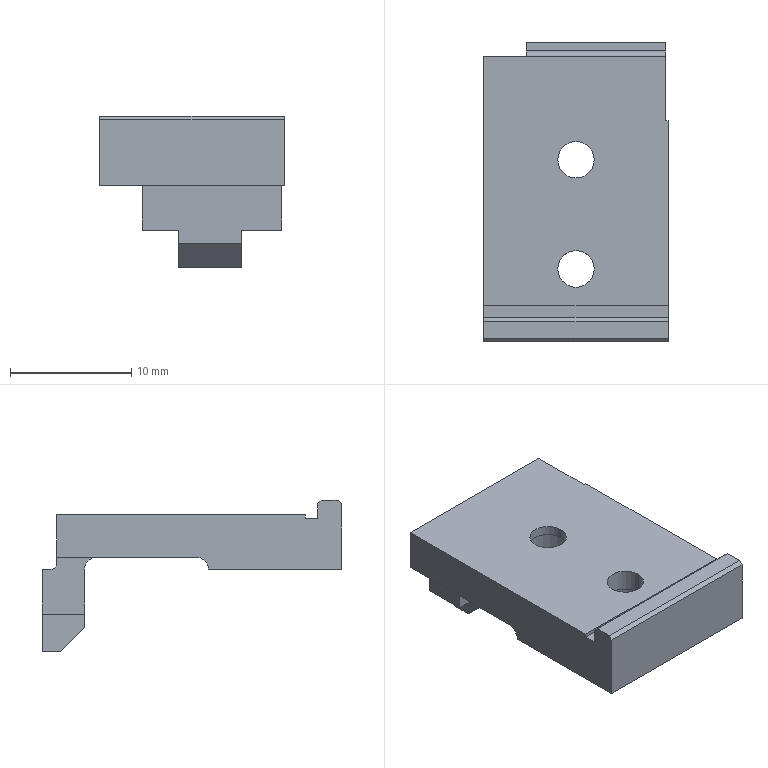Part | NX | 1 solid | 39 faces | box 15.2 x 24.7 x 12.5 mm | volume 1547 mm3 | plane 28 | cylinder 11 | commonest cylinder face diameters 3 x4 5 x4 2 x2 1 x1
STEP:
#1=CARTESIAN_POINT('',(-15.2,-12.7,1.));
#2=VERTEX_POINT('',#1);
#3=CARTESIAN_POINT('',(-15.2,-1.2,1.));
#4=VERTEX_POINT('',#3);
#5=CARTESIAN_POINT('',(-15.2,0.,1.));
#6=DIRECTION('',(0.,1.,0.));
#7=VECTOR('',#6,1000.);
#8=LINE('',#5,#7);
#9=EDGE_CURVE('',#2,#4,#8,.T.);
#10=ORIENTED_EDGE('',*,*,#9,.F.);
#11=CARTESIAN_POINT('',(-15.2,-13.7,0.));
#12=VERTEX_POINT('',#11);
#13=CARTESIAN_POINT('',(-15.2,-12.7,0.));
#14=DIRECTION('',(1.,0.,0.));
#15=DIRECTION('',(0.,-1.,0.));
#16=AXIS2_PLACEMENT_3D('',#13,#14,#15);
#17=CIRCLE('',#16,1.);
#18=EDGE_CURVE('',#2,#12,#17,.T.);
#19=ORIENTED_EDGE('',*,*,#18,.T.);
#20=CARTESIAN_POINT('',(-15.2,-24.7,0.));
#21=VERTEX_POINT('',#20);
#22=CARTESIAN_POINT('',(-15.2,0.,0.));
#23=DIRECTION('',(0.,1.,0.));
#24=VECTOR('',#23,1000.);
#25=LINE('',#22,#24);
#26=EDGE_CURVE('',#21,#12,#25,.T.);
#27=ORIENTED_EDGE('',*,*,#26,.F.);
#28=CARTESIAN_POINT('',(-15.2,-24.7,5.4));
#29=VERTEX_POINT('',#28);
#30=CARTESIAN_POINT('',(-15.2,-24.7,0.));
#31=DIRECTION('',(0.,0.,-1.));
#32=VECTOR('',#31,1000.);
#33=LINE('',#30,#32);
#34=EDGE_CURVE('',#29,#21,#33,.T.);
#35=ORIENTED_EDGE('',*,*,#34,.F.);
#36=CARTESIAN_POINT('',(-15.2,-24.4,5.7));
#37=VERTEX_POINT('',#36);
#38=CARTESIAN_POINT('',(-15.2,0.,30.1));
#39=DIRECTION('',(0.,0.7071,0.7071));
#40=VECTOR('',#39,1000.);
#41=LINE('',#38,#40);
#42=EDGE_CURVE('',#29,#37,#41,.T.);
#43=ORIENTED_EDGE('',*,*,#42,.T.);
#44=CARTESIAN_POINT('',(-15.2,-23.,5.7));
#45=VERTEX_POINT('',#44);
#46=CARTESIAN_POINT('',(-15.2,0.,5.7));
#47=DIRECTION('',(0.,1.,0.));
#48=VECTOR('',#47,1000.);
#49=LINE('',#46,#48);
#50=EDGE_CURVE('',#37,#45,#49,.T.);
#51=ORIENTED_EDGE('',*,*,#50,.T.);
#52=CARTESIAN_POINT('',(-15.2,-22.7,5.4));
#53=VERTEX_POINT('',#52);
#54=CARTESIAN_POINT('',(-15.2,0.,-17.3));
#55=DIRECTION('',(0.,-0.7071,0.7071));
#56=VECTOR('',#55,1000.);
#57=LINE('',#54,#56);
#58=EDGE_CURVE('',#53,#45,#57,.T.);
#59=ORIENTED_EDGE('',*,*,#58,.F.);
#60=CARTESIAN_POINT('',(-15.2,-22.7,4.2));
#61=VERTEX_POINT('',#60);
#62=CARTESIAN_POINT('',(-15.2,-22.7,0.));
#63=DIRECTION('',(0.,0.,-1.));
#64=VECTOR('',#63,1000.);
#65=LINE('',#62,#64);
#66=EDGE_CURVE('',#53,#61,#65,.T.);
#67=ORIENTED_EDGE('',*,*,#66,.T.);
#68=CARTESIAN_POINT('',(-15.2,-21.7,4.2));
#69=VERTEX_POINT('',#68);
#70=CARTESIAN_POINT('',(-15.2,0.,4.2));
#71=DIRECTION('',(0.,-1.,0.));
#72=VECTOR('',#71,1000.);
#73=LINE('',#70,#72);
#74=EDGE_CURVE('',#69,#61,#73,.T.);
#75=ORIENTED_EDGE('',*,*,#74,.F.);
#76=CARTESIAN_POINT('',(-15.2,-21.7,4.5));
#77=VERTEX_POINT('',#76);
#78=CARTESIAN_POINT('',(-15.2,-21.7,0.));
#79=DIRECTION('',(0.,0.,-1.));
#80=VECTOR('',#79,1000.);
#81=LINE('',#78,#80);
#82=EDGE_CURVE('',#77,#69,#81,.T.);
#83=ORIENTED_EDGE('',*,*,#82,.F.);
#84=CARTESIAN_POINT('',(-15.2,-1.2,4.5));
#85=VERTEX_POINT('',#84);
#86=CARTESIAN_POINT('',(-15.2,0.,4.5));
#87=DIRECTION('',(0.,-1.,0.));
#88=VECTOR('',#87,1000.);
#89=LINE('',#86,#88);
#90=EDGE_CURVE('',#85,#77,#89,.T.);
#91=ORIENTED_EDGE('',*,*,#90,.F.);
#92=CARTESIAN_POINT('',(-15.2,-1.2,0.));
#93=DIRECTION('',(0.,0.,1.));
#94=VECTOR('',#93,1000.);
#95=LINE('',#92,#94);
#96=EDGE_CURVE('',#4,#85,#95,.T.);
#97=ORIENTED_EDGE('',*,*,#96,.F.);
#98=EDGE_LOOP('',(#10,#19,#27,#35,#43,#51,#59,#67,#75,#83,#91,#97));
#99=FACE_BOUND('',#98,.T.);
#100=CARTESIAN_POINT('',(-15.2,0.,0.));
#101=DIRECTION('',(1.,0.,0.));
#102=DIRECTION('',(0.,1.,0.));
#103=AXIS2_PLACEMENT_3D('',#100,#101,#102);
#104=PLANE('',#103);
#105=ADVANCED_FACE('',(#99),#104,.F.);
#106=CARTESIAN_POINT('',(0.,-21.7,4.5));
#107=VERTEX_POINT('',#106);
#108=CARTESIAN_POINT('',(0.,-6.5,4.5));
#109=VERTEX_POINT('',#108);
#110=CARTESIAN_POINT('',(0.,0.,4.5));
#111=DIRECTION('',(0.,1.,0.));
#112=VECTOR('',#111,1000.);
#113=LINE('',#110,#112);
#114=EDGE_CURVE('',#107,#109,#113,.T.);
#115=ORIENTED_EDGE('',*,*,#114,.F.);
#116=CARTESIAN_POINT('',(0.,-21.7,4.2));
#117=VERTEX_POINT('',#116);
#118=CARTESIAN_POINT('',(0.,-21.7,0.));
#119=DIRECTION('',(0.,0.,1.));
#120=VECTOR('',#119,1000.);
#121=LINE('',#118,#120);
#122=EDGE_CURVE('',#117,#107,#121,.T.);
#123=ORIENTED_EDGE('',*,*,#122,.F.);
#124=CARTESIAN_POINT('',(0.,-22.7,4.2));
#125=VERTEX_POINT('',#124);
#126=CARTESIAN_POINT('',(0.,0.,4.2));
#127=DIRECTION('',(0.,1.,0.));
#128=VECTOR('',#127,1000.);
#129=LINE('',#126,#128);
#130=EDGE_CURVE('',#125,#117,#129,.T.);
#131=ORIENTED_EDGE('',*,*,#130,.F.);
#132=CARTESIAN_POINT('',(0.,-22.7,5.4));
#133=VERTEX_POINT('',#132);
#134=CARTESIAN_POINT('',(0.,-22.7,0.));
#135=DIRECTION('',(0.,0.,1.));
#136=VECTOR('',#135,1000.);
#137=LINE('',#134,#136);
#138=EDGE_CURVE('',#125,#133,#137,.T.);
#139=ORIENTED_EDGE('',*,*,#138,.T.);
#140=CARTESIAN_POINT('',(0.,-23.,5.7));
#141=VERTEX_POINT('',#140);
#142=CARTESIAN_POINT('',(0.,0.,-17.3));
#143=DIRECTION('',(0.,0.7071,-0.7071));
#144=VECTOR('',#143,1000.);
#145=LINE('',#142,#144);
#146=EDGE_CURVE('',#141,#133,#145,.T.);
#147=ORIENTED_EDGE('',*,*,#146,.F.);
#148=CARTESIAN_POINT('',(0.,-24.4,5.7));
#149=VERTEX_POINT('',#148);
#150=CARTESIAN_POINT('',(0.,0.,5.7));
#151=DIRECTION('',(0.,-1.,0.));
#152=VECTOR('',#151,1000.);
#153=LINE('',#150,#152);
#154=EDGE_CURVE('',#141,#149,#153,.T.);
#155=ORIENTED_EDGE('',*,*,#154,.T.);
#156=CARTESIAN_POINT('',(0.,-24.7,5.4));
#157=VERTEX_POINT('',#156);
#158=CARTESIAN_POINT('',(0.,0.,30.1));
#159=DIRECTION('',(0.,-0.7071,-0.7071));
#160=VECTOR('',#159,1000.);
#161=LINE('',#158,#160);
#162=EDGE_CURVE('',#149,#157,#161,.T.);
#163=ORIENTED_EDGE('',*,*,#162,.T.);
#164=CARTESIAN_POINT('',(0.,-24.7,0.));
#165=VERTEX_POINT('',#164);
#166=CARTESIAN_POINT('',(0.,-24.7,0.));
#167=DIRECTION('',(0.,0.,1.));
#168=VECTOR('',#167,1000.);
#169=LINE('',#166,#168);
#170=EDGE_CURVE('',#165,#157,#169,.T.);
#171=ORIENTED_EDGE('',*,*,#170,.F.);
#172=CARTESIAN_POINT('',(0.,-13.7,0.));
#173=VERTEX_POINT('',#172);
#174=CARTESIAN_POINT('',(0.,0.,0.));
#175=DIRECTION('',(0.,-1.,0.));
#176=VECTOR('',#175,1000.);
#177=LINE('',#174,#176);
#178=EDGE_CURVE('',#173,#165,#177,.T.);
#179=ORIENTED_EDGE('',*,*,#178,.F.);
#180=CARTESIAN_POINT('',(0.,-12.7,1.));
#181=VERTEX_POINT('',#180);
#182=CARTESIAN_POINT('',(0.,-12.7,0.));
#183=DIRECTION('',(1.,0.,0.));
#184=DIRECTION('',(0.,-1.,0.));
#185=AXIS2_PLACEMENT_3D('',#182,#183,#184);
#186=CIRCLE('',#185,1.);
#187=EDGE_CURVE('',#181,#173,#186,.T.);
#188=ORIENTED_EDGE('',*,*,#187,.F.);
#189=CARTESIAN_POINT('',(0.,-6.5,1.));
#190=VERTEX_POINT('',#189);
#191=CARTESIAN_POINT('',(0.,0.,1.));
#192=DIRECTION('',(0.,-1.,0.));
#193=VECTOR('',#192,1000.);
#194=LINE('',#191,#193);
#195=EDGE_CURVE('',#190,#181,#194,.T.);
#196=ORIENTED_EDGE('',*,*,#195,.F.);
#197=CARTESIAN_POINT('',(0.,-6.5,0.));
#198=DIRECTION('',(0.,0.,-1.));
#199=VECTOR('',#198,1000.);
#200=LINE('',#197,#199);
#201=EDGE_CURVE('',#109,#190,#200,.T.);
#202=ORIENTED_EDGE('',*,*,#201,.F.);
#203=EDGE_LOOP('',(#115,#123,#131,#139,#147,#155,#163,#171,#179,#188,#196,#202));
#204=FACE_BOUND('',#203,.T.);
#205=CARTESIAN_POINT('',(0.,-24.7,0.));
#206=DIRECTION('',(-1.,0.,0.));
#207=DIRECTION('',(0.,0.,1.));
#208=AXIS2_PLACEMENT_3D('',#205,#206,#207);
#209=PLANE('',#208);
#210=ADVANCED_FACE('',(#204),#209,.F.);
#211=CARTESIAN_POINT('',(-0.2,-1.2,4.5));
#212=VERTEX_POINT('',#211);
#213=CARTESIAN_POINT('',(-0.2,-6.5,4.5));
#214=VERTEX_POINT('',#213);
#215=CARTESIAN_POINT('',(-0.2,0.,4.5));
#216=DIRECTION('',(0.,-1.,0.));
#217=VECTOR('',#216,1000.);
#218=LINE('',#215,#217);
#219=EDGE_CURVE('',#212,#214,#218,.T.);
#220=ORIENTED_EDGE('',*,*,#219,.F.);
#221=CARTESIAN_POINT('',(0.,-1.2,4.5));
#222=DIRECTION('',(1.,0.,0.));
#223=VECTOR('',#222,1000.);
#224=LINE('',#221,#223);
#225=EDGE_CURVE('',#85,#212,#224,.T.);
#226=ORIENTED_EDGE('',*,*,#225,.F.);
#227=ORIENTED_EDGE('',*,*,#90,.T.);
#228=CARTESIAN_POINT('',(0.,-21.7,4.5));
#229=DIRECTION('',(-1.,0.,0.));
#230=VECTOR('',#229,1000.);
#231=LINE('',#228,#230);
#232=EDGE_CURVE('',#107,#77,#231,.T.);
#233=ORIENTED_EDGE('',*,*,#232,.F.);
#234=ORIENTED_EDGE('',*,*,#114,.T.);
#235=CARTESIAN_POINT('',(0.,-6.5,4.5));
#236=DIRECTION('',(1.,0.,0.));
#237=VECTOR('',#236,1000.);
#238=LINE('',#235,#237);
#239=EDGE_CURVE('',#214,#109,#238,.T.);
#240=ORIENTED_EDGE('',*,*,#239,.F.);
#241=EDGE_LOOP('',(#220,#226,#227,#233,#234,#240));
#242=FACE_BOUND('',#241,.T.);
#243=CARTESIAN_POINT('',(-6.1,-9.7,4.5));
#244=VERTEX_POINT('',#243);
#245=CARTESIAN_POINT('',(-9.1,-9.7,4.5));
#246=VERTEX_POINT('',#245);
#247=CARTESIAN_POINT('',(-7.6,-9.7,4.5));
#248=DIRECTION('',(0.,0.,-1.));
#249=DIRECTION('',(-1.,0.,0.));
#250=AXIS2_PLACEMENT_3D('',#247,#248,#249);
#251=CIRCLE('',#250,1.5);
#252=EDGE_CURVE('',#244,#246,#251,.T.);
#253=ORIENTED_EDGE('',*,*,#252,.T.);
#254=CARTESIAN_POINT('',(-7.6,-9.7,4.5));
#255=DIRECTION('',(0.,0.,-1.));
#256=DIRECTION('',(-1.,0.,0.));
#257=AXIS2_PLACEMENT_3D('',#254,#255,#256);
#258=CIRCLE('',#257,1.5);
#259=EDGE_CURVE('',#246,#244,#258,.T.);
#260=ORIENTED_EDGE('',*,*,#259,.T.);
#261=EDGE_LOOP('',(#253,#260));
#262=FACE_BOUND('',#261,.T.);
#263=CARTESIAN_POINT('',(-9.1,-18.7,4.5));
#264=VERTEX_POINT('',#263);
#265=CARTESIAN_POINT('',(-6.1,-18.7,4.5));
#266=VERTEX_POINT('',#265);
#267=CARTESIAN_POINT('',(-7.6,-18.7,4.5));
#268=DIRECTION('',(0.,0.,-1.));
#269=DIRECTION('',(-1.,0.,0.));
#270=AXIS2_PLACEMENT_3D('',#267,#268,#269);
#271=CIRCLE('',#270,1.5);
#272=EDGE_CURVE('',#264,#266,#271,.T.);
#273=ORIENTED_EDGE('',*,*,#272,.T.);
#274=CARTESIAN_POINT('',(-7.6,-18.7,4.5));
#275=DIRECTION('',(0.,0.,-1.));
#276=DIRECTION('',(-1.,0.,0.));
#277=AXIS2_PLACEMENT_3D('',#274,#275,#276);
#278=CIRCLE('',#277,1.5);
#279=EDGE_CURVE('',#266,#264,#278,.T.);
#280=ORIENTED_EDGE('',*,*,#279,.T.);
#281=EDGE_LOOP('',(#273,#280));
#282=FACE_BOUND('',#281,.T.);
#283=CARTESIAN_POINT('',(0.,0.,4.5));
#284=DIRECTION('',(0.,0.,1.));
#285=DIRECTION('',(1.,0.,0.));
#286=AXIS2_PLACEMENT_3D('',#283,#284,#285);
#287=PLANE('',#286);
#288=ADVANCED_FACE('',(#242,#262,#282),#287,.T.);
#289=CARTESIAN_POINT('',(-0.2,-4.5,1.));
#290=VERTEX_POINT('',#289);
#291=CARTESIAN_POINT('',(-11.7,-4.5,1.));
#292=VERTEX_POINT('',#291);
#293=CARTESIAN_POINT('',(0.,-4.5,1.));
#294=DIRECTION('',(-1.,0.,0.));
#295=VECTOR('',#294,1000.);
#296=LINE('',#293,#295);
#297=EDGE_CURVE('',#290,#292,#296,.T.);
#298=ORIENTED_EDGE('',*,*,#297,.F.);
#299=CARTESIAN_POINT('',(-0.2,-6.5,1.));
#300=VERTEX_POINT('',#299);
#301=CARTESIAN_POINT('',(-0.2,0.,1.));
#302=DIRECTION('',(0.,-1.,0.));
#303=VECTOR('',#302,1000.);
#304=LINE('',#301,#303);
#305=EDGE_CURVE('',#290,#300,#304,.T.);
#306=ORIENTED_EDGE('',*,*,#305,.T.);
#307=CARTESIAN_POINT('',(0.,-6.5,1.));
#308=DIRECTION('',(-1.,0.,0.));
#309=VECTOR('',#308,1000.);
#310=LINE('',#307,#309);
#311=EDGE_CURVE('',#190,#300,#310,.T.);
#312=ORIENTED_EDGE('',*,*,#311,.F.);
#313=ORIENTED_EDGE('',*,*,#195,.T.);
#314=CARTESIAN_POINT('',(0.,-12.7,1.));
#315=DIRECTION('',(1.,0.,0.));
#316=VECTOR('',#315,1000.);
#317=LINE('',#314,#316);
#318=EDGE_CURVE('',#2,#181,#317,.T.);
#319=ORIENTED_EDGE('',*,*,#318,.F.);
#320=ORIENTED_EDGE('',*,*,#9,.T.);
#321=CARTESIAN_POINT('',(-11.7,-1.2,1.));
#322=VERTEX_POINT('',#321);
#323=CARTESIAN_POINT('',(0.,-1.2,1.));
#324=DIRECTION('',(-1.,0.,0.));
#325=VECTOR('',#324,1000.);
#326=LINE('',#323,#325);
#327=EDGE_CURVE('',#322,#4,#326,.T.);
#328=ORIENTED_EDGE('',*,*,#327,.F.);
#329=CARTESIAN_POINT('',(-11.7,0.,1.));
#330=DIRECTION('',(0.,-1.,0.));
#331=VECTOR('',#330,1000.);
#332=LINE('',#329,#331);
#333=EDGE_CURVE('',#322,#292,#332,.T.);
#334=ORIENTED_EDGE('',*,*,#333,.T.);
#335=EDGE_LOOP('',(#298,#306,#312,#313,#319,#320,#328,#334));
#336=FACE_BOUND('',#335,.T.);
#337=CARTESIAN_POINT('',(-5.1,-9.7,1.));
#338=VERTEX_POINT('',#337);
#339=CARTESIAN_POINT('',(-10.1,-9.7,1.));
#340=VERTEX_POINT('',#339);
#341=CARTESIAN_POINT('',(-7.6,-9.7,1.));
#342=DIRECTION('',(0.,0.,-1.));
#343=DIRECTION('',(-1.,0.,0.));
#344=AXIS2_PLACEMENT_3D('',#341,#342,#343);
#345=CIRCLE('',#344,2.5);
#346=EDGE_CURVE('',#338,#340,#345,.T.);
#347=ORIENTED_EDGE('',*,*,#346,.F.);
#348=CARTESIAN_POINT('',(-7.6,-9.7,1.));
#349=DIRECTION('',(0.,0.,-1.));
#350=DIRECTION('',(-1.,0.,0.));
#351=AXIS2_PLACEMENT_3D('',#348,#349,#350);
#352=CIRCLE('',#351,2.5);
#353=EDGE_CURVE('',#340,#338,#352,.T.);
#354=ORIENTED_EDGE('',*,*,#353,.F.);
#355=EDGE_LOOP('',(#347,#354));
#356=FACE_BOUND('',#355,.T.);
#357=CARTESIAN_POINT('',(-11.724,-4.43,1.));
#358=DIRECTION('',(0.,0.,-1.));
#359=DIRECTION('',(0.,-1.,0.));
#360=AXIS2_PLACEMENT_3D('',#357,#358,#359);
#361=PLANE('',#360);
#362=ADVANCED_FACE('',(#336,#356),#361,.T.);
#363=CARTESIAN_POINT('',(-0.2,-3.5,-3.7));
#364=VERTEX_POINT('',#363);
#365=CARTESIAN_POINT('',(-0.2,0.,-3.7));
#366=VERTEX_POINT('',#365);
#367=CARTESIAN_POINT('',(-0.2,0.,-3.7));
#368=DIRECTION('',(0.,1.,0.));
#369=VECTOR('',#368,1000.);
#370=LINE('',#367,#369);
#371=EDGE_CURVE('',#364,#366,#370,.T.);
#372=ORIENTED_EDGE('',*,*,#371,.T.);
#373=CARTESIAN_POINT('',(-0.2,0.,0.));
#374=VERTEX_POINT('',#373);
#375=CARTESIAN_POINT('',(-0.2,0.,0.));
#376=DIRECTION('',(0.,0.,-1.));
#377=VECTOR('',#376,1000.);
#378=LINE('',#375,#377);
#379=EDGE_CURVE('',#374,#366,#378,.T.);
#380=ORIENTED_EDGE('',*,*,#379,.F.);
#381=CARTESIAN_POINT('',(-0.2,-0.7,0.));
#382=VERTEX_POINT('',#381);
#383=CARTESIAN_POINT('',(-0.2,0.,0.));
#384=DIRECTION('',(0.,1.,0.));
#385=VECTOR('',#384,1000.);
#386=LINE('',#383,#385);
#387=EDGE_CURVE('',#382,#374,#386,.T.);
#388=ORIENTED_EDGE('',*,*,#387,.F.);
#389=CARTESIAN_POINT('',(-0.2,-1.2,0.5));
#390=VERTEX_POINT('',#389);
#391=CARTESIAN_POINT('',(-0.2,-0.7,0.5));
#392=DIRECTION('',(-1.,0.,0.));
#393=DIRECTION('',(0.,1.,0.));
#394=AXIS2_PLACEMENT_3D('',#391,#392,#393);
#395=CIRCLE('',#394,0.5);
#396=EDGE_CURVE('',#382,#390,#395,.T.);
#397=ORIENTED_EDGE('',*,*,#396,.T.);
#398=CARTESIAN_POINT('',(-0.2,-1.2,0.));
#399=DIRECTION('',(0.,0.,-1.));
#400=VECTOR('',#399,1000.);
#401=LINE('',#398,#400);
#402=EDGE_CURVE('',#212,#390,#401,.T.);
#403=ORIENTED_EDGE('',*,*,#402,.F.);
#404=ORIENTED_EDGE('',*,*,#219,.T.);
#405=CARTESIAN_POINT('',(-0.2,-6.5,0.));
#406=DIRECTION('',(0.,0.,-1.));
#407=VECTOR('',#406,1000.);
#408=LINE('',#405,#407);
#409=EDGE_CURVE('',#214,#300,#408,.T.);
#410=ORIENTED_EDGE('',*,*,#409,.T.);
#411=ORIENTED_EDGE('',*,*,#305,.F.);
#412=CARTESIAN_POINT('',(-0.2,-3.5,0.));
#413=VERTEX_POINT('',#412);
#414=CARTESIAN_POINT('',(-0.2,-4.5,0.));
#415=DIRECTION('',(-1.,0.,0.));
#416=DIRECTION('',(0.,1.,0.));
#417=AXIS2_PLACEMENT_3D('',#414,#415,#416);
#418=CIRCLE('',#417,1.);
#419=EDGE_CURVE('',#290,#413,#418,.T.);
#420=ORIENTED_EDGE('',*,*,#419,.T.);
#421=CARTESIAN_POINT('',(-0.2,-3.5,0.));
#422=DIRECTION('',(0.,0.,1.));
#423=VECTOR('',#422,1000.);
#424=LINE('',#421,#423);
#425=EDGE_CURVE('',#364,#413,#424,.T.);
#426=ORIENTED_EDGE('',*,*,#425,.F.);
#427=EDGE_LOOP('',(#372,#380,#388,#397,#403,#404,#410,#411,#420,#426));
#428=FACE_BOUND('',#427,.T.);
#429=CARTESIAN_POINT('',(-0.2,-6.5,2.));
#430=DIRECTION('',(1.,0.,0.));
#431=DIRECTION('',(0.,1.,0.));
#432=AXIS2_PLACEMENT_3D('',#429,#430,#431);
#433=PLANE('',#432);
#434=ADVANCED_FACE('',(#428),#433,.T.);
#435=ORIENTED_EDGE('',*,*,#82,.T.);
#436=CARTESIAN_POINT('',(0.,-21.7,4.2));
#437=DIRECTION('',(1.,0.,0.));
#438=VECTOR('',#437,1000.);
#439=LINE('',#436,#438);
#440=EDGE_CURVE('',#69,#117,#439,.T.);
#441=ORIENTED_EDGE('',*,*,#440,.T.);
#442=ORIENTED_EDGE('',*,*,#122,.T.);
#443=ORIENTED_EDGE('',*,*,#232,.T.);
#444=EDGE_LOOP('',(#435,#441,#442,#443));
#445=FACE_BOUND('',#444,.T.);
#446=CARTESIAN_POINT('',(0.,-21.7,2.));
#447=DIRECTION('',(0.,-1.,0.));
#448=DIRECTION('',(0.,0.,-1.));
#449=AXIS2_PLACEMENT_3D('',#446,#447,#448);
#450=PLANE('',#449);
#451=ADVANCED_FACE('',(#445),#450,.T.);
#452=CARTESIAN_POINT('',(-11.7,0.,-3.7));
#453=VERTEX_POINT('',#452);
#454=CARTESIAN_POINT('',(-11.7,-3.5,-3.7));
#455=VERTEX_POINT('',#454);
#456=CARTESIAN_POINT('',(-11.7,0.,-3.7));
#457=DIRECTION('',(0.,-1.,0.));
#458=VECTOR('',#457,1000.);
#459=LINE('',#456,#458);
#460=EDGE_CURVE('',#453,#455,#459,.T.);
#461=ORIENTED_EDGE('',*,*,#460,.T.);
#462=CARTESIAN_POINT('',(-11.7,-3.5,0.));
#463=VERTEX_POINT('',#462);
#464=CARTESIAN_POINT('',(-11.7,-3.5,0.));
#465=DIRECTION('',(0.,0.,1.));
#466=VECTOR('',#465,1000.);
#467=LINE('',#464,#466);
#468=EDGE_CURVE('',#455,#463,#467,.T.);
#469=ORIENTED_EDGE('',*,*,#468,.T.);
#470=CARTESIAN_POINT('',(-11.7,-4.5,0.));
#471=DIRECTION('',(-1.,0.,0.));
#472=DIRECTION('',(0.,1.,0.));
#473=AXIS2_PLACEMENT_3D('',#470,#471,#472);
#474=CIRCLE('',#473,1.);
#475=EDGE_CURVE('',#292,#463,#474,.T.);
#476=ORIENTED_EDGE('',*,*,#475,.F.);
#477=ORIENTED_EDGE('',*,*,#333,.F.);
#478=CARTESIAN_POINT('',(-11.7,-1.2,0.5));
#479=VERTEX_POINT('',#478);
#480=CARTESIAN_POINT('',(-11.7,-1.2,0.));
#481=DIRECTION('',(0.,0.,-1.));
#482=VECTOR('',#481,1000.);
#483=LINE('',#480,#482);
#484=EDGE_CURVE('',#322,#479,#483,.T.);
#485=ORIENTED_EDGE('',*,*,#484,.T.);
#486=CARTESIAN_POINT('',(-11.7,-0.7,0.));
#487=VERTEX_POINT('',#486);
#488=CARTESIAN_POINT('',(-11.7,-0.7,0.5));
#489=DIRECTION('',(-1.,0.,0.));
#490=DIRECTION('',(0.,1.,0.));
#491=AXIS2_PLACEMENT_3D('',#488,#489,#490);
#492=CIRCLE('',#491,0.5);
#493=EDGE_CURVE('',#487,#479,#492,.T.);
#494=ORIENTED_EDGE('',*,*,#493,.F.);
#495=CARTESIAN_POINT('',(-11.7,0.,0.));
#496=VERTEX_POINT('',#495);
#497=CARTESIAN_POINT('',(-11.7,0.,0.));
#498=DIRECTION('',(0.,1.,0.));
#499=VECTOR('',#498,1000.);
#500=LINE('',#497,#499);
#501=EDGE_CURVE('',#487,#496,#500,.T.);
#502=ORIENTED_EDGE('',*,*,#501,.T.);
#503=CARTESIAN_POINT('',(-11.7,0.,0.));
#504=DIRECTION('',(0.,0.,-1.));
#505=VECTOR('',#504,1000.);
#506=LINE('',#503,#505);
#507=EDGE_CURVE('',#496,#453,#506,.T.);
#508=ORIENTED_EDGE('',*,*,#507,.T.);
#509=EDGE_LOOP('',(#461,#469,#476,#477,#485,#494,#502,#508));
#510=FACE_BOUND('',#509,.T.);
#511=CARTESIAN_POINT('',(-11.7,-1.2,0.));
#512=DIRECTION('',(1.,0.,0.));
#513=DIRECTION('',(0.,1.,0.));
#514=AXIS2_PLACEMENT_3D('',#511,#512,#513);
#515=PLANE('',#514);
#516=ADVANCED_FACE('',(#510),#515,.F.);
#517=ORIENTED_EDGE('',*,*,#311,.T.);
#518=ORIENTED_EDGE('',*,*,#409,.F.);
#519=ORIENTED_EDGE('',*,*,#239,.T.);
#520=ORIENTED_EDGE('',*,*,#201,.T.);
#521=EDGE_LOOP('',(#517,#518,#519,#520));
#522=FACE_BOUND('',#521,.T.);
#523=CARTESIAN_POINT('',(0.,-6.5,2.));
#524=DIRECTION('',(0.,1.,0.));
#525=DIRECTION('',(1.,0.,0.));
#526=AXIS2_PLACEMENT_3D('',#523,#524,#525);
#527=PLANE('',#526);
#528=ADVANCED_FACE('',(#522),#527,.T.);
#529=CARTESIAN_POINT('',(-5.1,-18.7,2.7));
#530=VERTEX_POINT('',#529);
#531=CARTESIAN_POINT('',(-10.1,-18.7,2.7));
#532=VERTEX_POINT('',#531);
#533=CARTESIAN_POINT('',(-7.6,-18.7,2.7));
#534=DIRECTION('',(0.,0.,-1.));
#535=DIRECTION('',(-1.,0.,0.));
#536=AXIS2_PLACEMENT_3D('',#533,#534,#535);
#537=CIRCLE('',#536,2.5);
#538=EDGE_CURVE('',#530,#532,#537,.T.);
#539=ORIENTED_EDGE('',*,*,#538,.T.);
#540=CARTESIAN_POINT('',(-7.6,-18.7,2.7));
#541=DIRECTION('',(0.,0.,-1.));
#542=DIRECTION('',(-1.,0.,0.));
#543=AXIS2_PLACEMENT_3D('',#540,#541,#542);
#544=CIRCLE('',#543,2.5);
#545=EDGE_CURVE('',#532,#530,#544,.T.);
#546=ORIENTED_EDGE('',*,*,#545,.T.);
#547=EDGE_LOOP('',(#539,#546));
#548=FACE_BOUND('',#547,.T.);
#549=CARTESIAN_POINT('',(-6.1,-18.7,2.7));
#550=VERTEX_POINT('',#549);
#551=CARTESIAN_POINT('',(-9.1,-18.7,2.7));
#552=VERTEX_POINT('',#551);
#553=CARTESIAN_POINT('',(-7.6,-18.7,2.7));
#554=DIRECTION('',(0.,0.,-1.));
#555=DIRECTION('',(-1.,0.,0.));
#556=AXIS2_PLACEMENT_3D('',#553,#554,#555);
#557=CIRCLE('',#556,1.5);
#558=EDGE_CURVE('',#550,#552,#557,.T.);
#559=ORIENTED_EDGE('',*,*,#558,.F.);
#560=CARTESIAN_POINT('',(-7.6,-18.7,2.7));
#561=DIRECTION('',(0.,0.,-1.));
#562=DIRECTION('',(-1.,0.,0.));
#563=AXIS2_PLACEMENT_3D('',#560,#561,#562);
#564=CIRCLE('',#563,1.5);
#565=EDGE_CURVE('',#552,#550,#564,.T.);
#566=ORIENTED_EDGE('',*,*,#565,.F.);
#567=EDGE_LOOP('',(#559,#566));
#568=FACE_BOUND('',#567,.T.);
#569=CARTESIAN_POINT('',(-11.486,-5.492,2.7));
#570=DIRECTION('',(0.,0.,-1.));
#571=DIRECTION('',(0.,-1.,0.));
#572=AXIS2_PLACEMENT_3D('',#569,#570,#571);
#573=PLANE('',#572);
#574=ADVANCED_FACE('',(#548,#568),#573,.T.);
#575=ORIENTED_EDGE('',*,*,#387,.T.);
#576=CARTESIAN_POINT('',(0.,0.,0.));
#577=DIRECTION('',(1.,0.,0.));
#578=VECTOR('',#577,1000.);
#579=LINE('',#576,#578);
#580=EDGE_CURVE('',#496,#374,#579,.T.);
#581=ORIENTED_EDGE('',*,*,#580,.F.);
#582=ORIENTED_EDGE('',*,*,#501,.F.);
#583=CARTESIAN_POINT('',(0.,-0.7,0.));
#584=DIRECTION('',(-1.,0.,0.));
#585=VECTOR('',#584,1000.);
#586=LINE('',#583,#585);
#587=EDGE_CURVE('',#382,#487,#586,.T.);
#588=ORIENTED_EDGE('',*,*,#587,.F.);
#589=EDGE_LOOP('',(#575,#581,#582,#588));
#590=FACE_BOUND('',#589,.T.);
#591=CARTESIAN_POINT('',(-15.2,-1.2,0.));
#592=DIRECTION('',(0.,0.,1.));
#593=DIRECTION('',(1.,0.,0.));
#594=AXIS2_PLACEMENT_3D('',#591,#592,#593);
#595=PLANE('',#594);
#596=ADVANCED_FACE('',(#590),#595,.T.);
#597=CARTESIAN_POINT('',(-4.1,0.,-6.8));
#598=VERTEX_POINT('',#597);
#599=CARTESIAN_POINT('',(-4.1,0.,-3.7));
#600=VERTEX_POINT('',#599);
#601=CARTESIAN_POINT('',(-4.1,0.,0.));
#602=DIRECTION('',(0.,0.,1.));
#603=VECTOR('',#602,1000.);
#604=LINE('',#601,#603);
#605=EDGE_CURVE('',#598,#600,#604,.T.);
#606=ORIENTED_EDGE('',*,*,#605,.F.);
#607=CARTESIAN_POINT('',(-8.7,0.,-6.8));
#608=VERTEX_POINT('',#607);
#609=CARTESIAN_POINT('',(0.,0.,-6.8));
#610=DIRECTION('',(-1.,0.,0.));
#611=VECTOR('',#610,1000.);
#612=LINE('',#609,#611);
#613=EDGE_CURVE('',#598,#608,#612,.T.);
#614=ORIENTED_EDGE('',*,*,#613,.T.);
#615=CARTESIAN_POINT('',(-8.7,0.,-3.7));
#616=VERTEX_POINT('',#615);
#617=CARTESIAN_POINT('',(-8.7,0.,0.));
#618=DIRECTION('',(0.,0.,1.));
#619=VECTOR('',#618,1000.);
#620=LINE('',#617,#619);
#621=EDGE_CURVE('',#608,#616,#620,.T.);
#622=ORIENTED_EDGE('',*,*,#621,.T.);
#623=CARTESIAN_POINT('',(0.,0.,-3.7));
#624=DIRECTION('',(1.,0.,0.));
#625=VECTOR('',#624,1000.);
#626=LINE('',#623,#625);
#627=EDGE_CURVE('',#453,#616,#626,.T.);
#628=ORIENTED_EDGE('',*,*,#627,.F.);
#629=ORIENTED_EDGE('',*,*,#507,.F.);
#630=ORIENTED_EDGE('',*,*,#580,.T.);
#631=ORIENTED_EDGE('',*,*,#379,.T.);
#632=CARTESIAN_POINT('',(0.,0.,-3.7));
#633=DIRECTION('',(1.,0.,0.));
#634=VECTOR('',#633,1000.);
#635=LINE('',#632,#634);
#636=EDGE_CURVE('',#600,#366,#635,.T.);
#637=ORIENTED_EDGE('',*,*,#636,.F.);
#638=EDGE_LOOP('',(#606,#614,#622,#628,#629,#630,#631,#637));
#639=FACE_BOUND('',#638,.T.);
#640=CARTESIAN_POINT('',(0.,0.,0.));
#641=DIRECTION('',(0.,-1.,0.));
#642=DIRECTION('',(0.,0.,-1.));
#643=AXIS2_PLACEMENT_3D('',#640,#641,#642);
#644=PLANE('',#643);
#645=ADVANCED_FACE('',(#639),#644,.F.);
#646=CARTESIAN_POINT('',(-8.7,-3.5,-3.7));
#647=VERTEX_POINT('',#646);
#648=CARTESIAN_POINT('',(-8.7,-3.5,-4.8));
#649=VERTEX_POINT('',#648);
#650=CARTESIAN_POINT('',(-8.7,-3.5,0.));
#651=DIRECTION('',(0.,0.,-1.));
#652=VECTOR('',#651,1000.);
#653=LINE('',#650,#652);
#654=EDGE_CURVE('',#647,#649,#653,.T.);
#655=ORIENTED_EDGE('',*,*,#654,.F.);
#656=CARTESIAN_POINT('',(-8.7,0.,-3.7));
#657=DIRECTION('',(0.,1.,0.));
#658=VECTOR('',#657,1000.);
#659=LINE('',#656,#658);
#660=EDGE_CURVE('',#647,#616,#659,.T.);
#661=ORIENTED_EDGE('',*,*,#660,.T.);
#662=ORIENTED_EDGE('',*,*,#621,.F.);
#663=CARTESIAN_POINT('',(-8.7,-1.5,-6.8));
#664=VERTEX_POINT('',#663);
#665=CARTESIAN_POINT('',(-8.7,0.,-6.8));
#666=DIRECTION('',(0.,1.,0.));
#667=VECTOR('',#666,1000.);
#668=LINE('',#665,#667);
#669=EDGE_CURVE('',#664,#608,#668,.T.);
#670=ORIENTED_EDGE('',*,*,#669,.F.);
#671=CARTESIAN_POINT('',(-8.7,-8.3,0.));
#672=DIRECTION('',(0.,-0.7071,0.7071));
#673=VECTOR('',#672,1000.);
#674=LINE('',#671,#673);
#675=EDGE_CURVE('',#664,#649,#674,.T.);
#676=ORIENTED_EDGE('',*,*,#675,.T.);
#677=EDGE_LOOP('',(#655,#661,#662,#670,#676));
#678=FACE_BOUND('',#677,.T.);
#679=CARTESIAN_POINT('',(-8.7,2.4,-3.7));
#680=DIRECTION('',(-1.,0.,0.));
#681=DIRECTION('',(0.,0.,1.));
#682=AXIS2_PLACEMENT_3D('',#679,#680,#681);
#683=PLANE('',#682);
#684=ADVANCED_FACE('',(#678),#683,.T.);
#685=CARTESIAN_POINT('',(0.,-22.7,4.2));
#686=DIRECTION('',(1.,0.,0.));
#687=VECTOR('',#686,1000.);
#688=LINE('',#685,#687);
#689=EDGE_CURVE('',#61,#125,#688,.T.);
#690=ORIENTED_EDGE('',*,*,#689,.T.);
#691=ORIENTED_EDGE('',*,*,#130,.T.);
#692=ORIENTED_EDGE('',*,*,#440,.F.);
#693=ORIENTED_EDGE('',*,*,#74,.T.);
#694=EDGE_LOOP('',(#690,#691,#692,#693));
#695=FACE_BOUND('',#694,.T.);
#696=CARTESIAN_POINT('',(0.,-21.7,4.2));
#697=DIRECTION('',(0.,0.,1.));
#698=DIRECTION('',(1.,0.,0.));
#699=AXIS2_PLACEMENT_3D('',#696,#697,#698);
#700=PLANE('',#699);
#701=ADVANCED_FACE('',(#695),#700,.T.);
#702=CARTESIAN_POINT('',(-3.5,-1.5,-6.8));
#703=VERTEX_POINT('',#702);
#704=CARTESIAN_POINT('',(0.,-1.5,-6.8));
#705=DIRECTION('',(-1.,0.,0.));
#706=VECTOR('',#705,1000.);
#707=LINE('',#704,#706);
#708=EDGE_CURVE('',#703,#664,#707,.T.);
#709=ORIENTED_EDGE('',*,*,#708,.T.);
#710=ORIENTED_EDGE('',*,*,#669,.T.);
#711=ORIENTED_EDGE('',*,*,#613,.F.);
#712=CARTESIAN_POINT('',(-3.5,-0.3,-6.8));
#713=VERTEX_POINT('',#712);
#714=CARTESIAN_POINT('',(0.,-2.05,-6.8));
#715=DIRECTION('',(-0.8944,0.4472,0.));
#716=VECTOR('',#715,1000.);
#717=LINE('',#714,#716);
#718=EDGE_CURVE('',#713,#598,#717,.T.);
#719=ORIENTED_EDGE('',*,*,#718,.F.);
#720=CARTESIAN_POINT('',(-3.5,0.,-6.8));
#721=DIRECTION('',(0.,1.,0.));
#722=VECTOR('',#721,1000.);
#723=LINE('',#720,#722);
#724=EDGE_CURVE('',#703,#713,#723,.T.);
#725=ORIENTED_EDGE('',*,*,#724,.F.);
#726=EDGE_LOOP('',(#709,#710,#711,#719,#725));
#727=FACE_BOUND('',#726,.T.);
#728=CARTESIAN_POINT('',(-4.459,-2.381,-6.8));
#729=DIRECTION('',(0.,0.,-1.));
#730=DIRECTION('',(0.,-1.,0.));
#731=AXIS2_PLACEMENT_3D('',#728,#729,#730);
#732=PLANE('',#731);
#733=ADVANCED_FACE('',(#727),#732,.T.);
#734=CARTESIAN_POINT('',(0.,-1.2,0.5));
#735=DIRECTION('',(-1.,0.,0.));
#736=VECTOR('',#735,1000.);
#737=LINE('',#734,#736);
#738=EDGE_CURVE('',#390,#479,#737,.T.);
#739=ORIENTED_EDGE('',*,*,#738,.T.);
#740=ORIENTED_EDGE('',*,*,#484,.F.);
#741=ORIENTED_EDGE('',*,*,#327,.T.);
#742=ORIENTED_EDGE('',*,*,#96,.T.);
#743=ORIENTED_EDGE('',*,*,#225,.T.);
#744=ORIENTED_EDGE('',*,*,#402,.T.);
#745=EDGE_LOOP('',(#739,#740,#741,#742,#743,#744));
#746=FACE_BOUND('',#745,.T.);
#747=CARTESIAN_POINT('',(-15.2,-1.2,2.));
#748=DIRECTION('',(0.,1.,0.));
#749=DIRECTION('',(1.,0.,0.));
#750=AXIS2_PLACEMENT_3D('',#747,#748,#749);
#751=PLANE('',#750);
#752=ADVANCED_FACE('',(#746),#751,.T.);
#753=ORIENTED_EDGE('',*,*,#318,.T.);
#754=ORIENTED_EDGE('',*,*,#187,.T.);
#755=CARTESIAN_POINT('',(0.,-13.7,0.));
#756=DIRECTION('',(1.,0.,0.));
#757=VECTOR('',#756,1000.);
#758=LINE('',#755,#757);
#759=EDGE_CURVE('',#12,#173,#758,.T.);
#760=ORIENTED_EDGE('',*,*,#759,.F.);
#761=ORIENTED_EDGE('',*,*,#18,.F.);
#762=EDGE_LOOP('',(#753,#754,#760,#761));
#763=FACE_BOUND('',#762,.T.);
#764=CARTESIAN_POINT('',(0.,-12.7,0.));
#765=DIRECTION('',(1.,0.,0.));
#766=DIRECTION('',(0.,-1.,0.));
#767=AXIS2_PLACEMENT_3D('',#764,#765,#766);
#768=CYLINDRICAL_SURFACE('',#767,1.);
#769=ADVANCED_FACE('',(#763),#768,.F.);
#770=CARTESIAN_POINT('',(0.,-23.,5.7));
#771=DIRECTION('',(-1.,0.,0.));
#772=VECTOR('',#771,1000.);
#773=LINE('',#770,#772);
#774=EDGE_CURVE('',#141,#45,#773,.T.);
#775=ORIENTED_EDGE('',*,*,#774,.T.);
#776=ORIENTED_EDGE('',*,*,#50,.F.);
#777=CARTESIAN_POINT('',(0.,-24.4,5.7));
#778=DIRECTION('',(-1.,0.,0.));
#779=VECTOR('',#778,1000.);
#780=LINE('',#777,#779);
#781=EDGE_CURVE('',#149,#37,#780,.T.);
#782=ORIENTED_EDGE('',*,*,#781,.F.);
#783=ORIENTED_EDGE('',*,*,#154,.F.);
#784=EDGE_LOOP('',(#775,#776,#782,#783));
#785=FACE_BOUND('',#784,.T.);
#786=CARTESIAN_POINT('',(0.,-22.7,5.7));
#787=DIRECTION('',(0.,0.,-1.));
#788=DIRECTION('',(0.,-1.,0.));
#789=AXIS2_PLACEMENT_3D('',#786,#787,#788);
#790=PLANE('',#789);
#791=ADVANCED_FACE('',(#785),#790,.F.);
#792=ORIENTED_EDGE('',*,*,#689,.F.);
#793=ORIENTED_EDGE('',*,*,#66,.F.);
#794=CARTESIAN_POINT('',(0.,-22.7,5.4));
#795=DIRECTION('',(1.,0.,0.));
#796=VECTOR('',#795,1000.);
#797=LINE('',#794,#796);
#798=EDGE_CURVE('',#53,#133,#797,.T.);
#799=ORIENTED_EDGE('',*,*,#798,.T.);
#800=ORIENTED_EDGE('',*,*,#138,.F.);
#801=EDGE_LOOP('',(#792,#793,#799,#800));
#802=FACE_BOUND('',#801,.T.);
#803=CARTESIAN_POINT('',(0.,-22.7,2.));
#804=DIRECTION('',(0.,-1.,0.));
#805=DIRECTION('',(0.,0.,-1.));
#806=AXIS2_PLACEMENT_3D('',#803,#804,#805);
#807=PLANE('',#806);
#808=ADVANCED_FACE('',(#802),#807,.F.);
#809=ORIENTED_EDGE('',*,*,#774,.F.);
#810=ORIENTED_EDGE('',*,*,#146,.T.);
#811=ORIENTED_EDGE('',*,*,#798,.F.);
#812=ORIENTED_EDGE('',*,*,#58,.T.);
#813=EDGE_LOOP('',(#809,#810,#811,#812));
#814=FACE_BOUND('',#813,.T.);
#815=CARTESIAN_POINT('',(-7.6,-22.85,5.55));
#816=DIRECTION('',(0.,0.7071,0.7071));
#817=DIRECTION('',(1.,0.,0.));
#818=AXIS2_PLACEMENT_3D('',#815,#816,#817);
#819=PLANE('',#818);
#820=ADVANCED_FACE('',(#814),#819,.T.);
#821=CARTESIAN_POINT('',(-5.1,-18.7,0.));
#822=VERTEX_POINT('',#821);
#823=CARTESIAN_POINT('',(-10.1,-18.7,0.));
#824=VERTEX_POINT('',#823);
#825=CARTESIAN_POINT('',(-7.6,-18.7,0.));
#826=DIRECTION('',(0.,0.,-1.));
#827=DIRECTION('',(-1.,0.,0.));
#828=AXIS2_PLACEMENT_3D('',#825,#826,#827);
#829=CIRCLE('',#828,2.5);
#830=EDGE_CURVE('',#822,#824,#829,.T.);
#831=ORIENTED_EDGE('',*,*,#830,.T.);
#832=CARTESIAN_POINT('',(-10.1,-18.7,0.));
#833=DIRECTION('',(0.,0.,-1.));
#834=VECTOR('',#833,1000.);
#835=LINE('',#832,#834);
#836=EDGE_CURVE('',#824,#532,#835,.F.);
#837=ORIENTED_EDGE('',*,*,#836,.T.);
#838=ORIENTED_EDGE('',*,*,#538,.F.);
#839=CARTESIAN_POINT('',(-5.1,-18.7,0.));
#840=DIRECTION('',(0.,0.,-1.));
#841=VECTOR('',#840,1000.);
#842=LINE('',#839,#841);
#843=EDGE_CURVE('',#822,#530,#842,.F.);
#844=ORIENTED_EDGE('',*,*,#843,.F.);
#845=EDGE_LOOP('',(#831,#837,#838,#844));
#846=FACE_BOUND('',#845,.T.);
#847=CARTESIAN_POINT('',(-7.6,-18.7,0.));
#848=DIRECTION('',(0.,0.,-1.));
#849=DIRECTION('',(-1.,0.,0.));
#850=AXIS2_PLACEMENT_3D('',#847,#848,#849);
#851=CYLINDRICAL_SURFACE('',#850,2.5);
#852=ADVANCED_FACE('',(#846),#851,.F.);
#853=CARTESIAN_POINT('',(-5.1,-9.7,3.7));
#854=VERTEX_POINT('',#853);
#855=CARTESIAN_POINT('',(-10.1,-9.7,3.7));
#856=VERTEX_POINT('',#855);
#857=CARTESIAN_POINT('',(-7.6,-9.7,3.7));
#858=DIRECTION('',(0.,0.,-1.));
#859=DIRECTION('',(-1.,0.,0.));
#860=AXIS2_PLACEMENT_3D('',#857,#858,#859);
#861=CIRCLE('',#860,2.5);
#862=EDGE_CURVE('',#854,#856,#861,.T.);
#863=ORIENTED_EDGE('',*,*,#862,.F.);
#864=CARTESIAN_POINT('',(-5.1,-9.7,0.));
#865=DIRECTION('',(0.,0.,-1.));
#866=VECTOR('',#865,1000.);
#867=LINE('',#864,#866);
#868=EDGE_CURVE('',#338,#854,#867,.F.);
#869=ORIENTED_EDGE('',*,*,#868,.F.);
#870=ORIENTED_EDGE('',*,*,#346,.T.);
#871=CARTESIAN_POINT('',(-10.1,-9.7,0.));
#872=DIRECTION('',(0.,0.,-1.));
#873=VECTOR('',#872,1000.);
#874=LINE('',#871,#873);
#875=EDGE_CURVE('',#340,#856,#874,.F.);
#876=ORIENTED_EDGE('',*,*,#875,.T.);
#877=EDGE_LOOP('',(#863,#869,#870,#876));
#878=FACE_BOUND('',#877,.T.);
#879=CARTESIAN_POINT('',(-7.6,-9.7,0.));
#880=DIRECTION('',(0.,0.,-1.));
#881=DIRECTION('',(-1.,0.,0.));
#882=AXIS2_PLACEMENT_3D('',#879,#880,#881);
#883=CYLINDRICAL_SURFACE('',#882,2.5);
#884=ADVANCED_FACE('',(#878),#883,.F.);
#885=CARTESIAN_POINT('',(0.,-24.7,5.4));
#886=DIRECTION('',(1.,0.,0.));
#887=VECTOR('',#886,1000.);
#888=LINE('',#885,#887);
#889=EDGE_CURVE('',#29,#157,#888,.T.);
#890=ORIENTED_EDGE('',*,*,#889,.T.);
#891=ORIENTED_EDGE('',*,*,#162,.F.);
#892=ORIENTED_EDGE('',*,*,#781,.T.);
#893=ORIENTED_EDGE('',*,*,#42,.F.);
#894=EDGE_LOOP('',(#890,#891,#892,#893));
#895=FACE_BOUND('',#894,.T.);
#896=CARTESIAN_POINT('',(-7.6,-24.55,5.55));
#897=DIRECTION('',(0.,0.7071,-0.7071));
#898=DIRECTION('',(-1.,0.,0.));
#899=AXIS2_PLACEMENT_3D('',#896,#897,#898);
#900=PLANE('',#899);
#901=ADVANCED_FACE('',(#895),#900,.F.);
#902=ORIENTED_EDGE('',*,*,#252,.F.);
#903=CARTESIAN_POINT('',(-6.1,-9.7,3.7));
#904=VERTEX_POINT('',#903);
#905=CARTESIAN_POINT('',(-6.1,-9.7,5.45));
#906=DIRECTION('',(0.,0.,-1.));
#907=VECTOR('',#906,1000.);
#908=LINE('',#905,#907);
#909=EDGE_CURVE('',#244,#904,#908,.T.);
#910=ORIENTED_EDGE('',*,*,#909,.T.);
#911=CARTESIAN_POINT('',(-9.1,-9.7,3.7));
#912=VERTEX_POINT('',#911);
#913=CARTESIAN_POINT('',(-7.6,-9.7,3.7));
#914=DIRECTION('',(0.,0.,-1.));
#915=DIRECTION('',(-1.,0.,0.));
#916=AXIS2_PLACEMENT_3D('',#913,#914,#915);
#917=CIRCLE('',#916,1.5);
#918=EDGE_CURVE('',#904,#912,#917,.T.);
#919=ORIENTED_EDGE('',*,*,#918,.T.);
#920=CARTESIAN_POINT('',(-9.1,-9.7,5.45));
#921=DIRECTION('',(0.,0.,-1.));
#922=VECTOR('',#921,1000.);
#923=LINE('',#920,#922);
#924=EDGE_CURVE('',#246,#912,#923,.T.);
#925=ORIENTED_EDGE('',*,*,#924,.F.);
#926=EDGE_LOOP('',(#902,#910,#919,#925));
#927=FACE_BOUND('',#926,.T.);
#928=CARTESIAN_POINT('',(-7.6,-9.7,5.45));
#929=DIRECTION('',(0.,0.,-1.));
#930=DIRECTION('',(-1.,0.,0.));
#931=AXIS2_PLACEMENT_3D('',#928,#929,#930);
#932=CYLINDRICAL_SURFACE('',#931,1.5);
#933=ADVANCED_FACE('',(#927),#932,.F.);
#934=ORIENTED_EDGE('',*,*,#558,.T.);
#935=CARTESIAN_POINT('',(-9.1,-18.7,5.45));
#936=DIRECTION('',(0.,0.,-1.));
#937=VECTOR('',#936,1000.);
#938=LINE('',#935,#937);
#939=EDGE_CURVE('',#552,#264,#938,.F.);
#940=ORIENTED_EDGE('',*,*,#939,.T.);
#941=ORIENTED_EDGE('',*,*,#279,.F.);
#942=CARTESIAN_POINT('',(-6.1,-18.7,5.45));
#943=DIRECTION('',(0.,0.,-1.));
#944=VECTOR('',#943,1000.);
#945=LINE('',#942,#944);
#946=EDGE_CURVE('',#550,#266,#945,.F.);
#947=ORIENTED_EDGE('',*,*,#946,.F.);
#948=EDGE_LOOP('',(#934,#940,#941,#947));
#949=FACE_BOUND('',#948,.T.);
#950=CARTESIAN_POINT('',(-7.6,-18.7,5.45));
#951=DIRECTION('',(0.,0.,-1.));
#952=DIRECTION('',(-1.,0.,0.));
#953=AXIS2_PLACEMENT_3D('',#950,#951,#952);
#954=CYLINDRICAL_SURFACE('',#953,1.5);
#955=ADVANCED_FACE('',(#949),#954,.F.);
#956=ORIENTED_EDGE('',*,*,#759,.T.);
#957=ORIENTED_EDGE('',*,*,#178,.T.);
#958=CARTESIAN_POINT('',(0.,-24.7,0.));
#959=DIRECTION('',(1.,0.,0.));
#960=VECTOR('',#959,1000.);
#961=LINE('',#958,#960);
#962=EDGE_CURVE('',#21,#165,#961,.T.);
#963=ORIENTED_EDGE('',*,*,#962,.F.);
#964=ORIENTED_EDGE('',*,*,#26,.T.);
#965=EDGE_LOOP('',(#956,#957,#963,#964));
#966=FACE_BOUND('',#965,.T.);
#967=ORIENTED_EDGE('',*,*,#830,.F.);
#968=CARTESIAN_POINT('',(-7.6,-18.7,0.));
#969=DIRECTION('',(0.,0.,-1.));
#970=DIRECTION('',(-1.,0.,0.));
#971=AXIS2_PLACEMENT_3D('',#968,#969,#970);
#972=CIRCLE('',#971,2.5);
#973=EDGE_CURVE('',#824,#822,#972,.T.);
#974=ORIENTED_EDGE('',*,*,#973,.F.);
#975=EDGE_LOOP('',(#967,#974));
#976=FACE_BOUND('',#975,.T.);
#977=CARTESIAN_POINT('',(-11.977,-15.053,0.));
#978=DIRECTION('',(0.,0.,-1.));
#979=DIRECTION('',(0.,-1.,0.));
#980=AXIS2_PLACEMENT_3D('',#977,#978,#979);
#981=PLANE('',#980);
#982=ADVANCED_FACE('',(#966,#976),#981,.T.);
#983=ORIENTED_EDGE('',*,*,#862,.T.);
#984=CARTESIAN_POINT('',(-7.6,-9.7,3.7));
#985=DIRECTION('',(0.,0.,-1.));
#986=DIRECTION('',(-1.,0.,0.));
#987=AXIS2_PLACEMENT_3D('',#984,#985,#986);
#988=CIRCLE('',#987,2.5);
#989=EDGE_CURVE('',#856,#854,#988,.T.);
#990=ORIENTED_EDGE('',*,*,#989,.T.);
#991=EDGE_LOOP('',(#983,#990));
#992=FACE_BOUND('',#991,.T.);
#993=CARTESIAN_POINT('',(-7.6,-9.7,3.7));
#994=DIRECTION('',(0.,0.,-1.));
#995=DIRECTION('',(-1.,0.,0.));
#996=AXIS2_PLACEMENT_3D('',#993,#994,#995);
#997=CIRCLE('',#996,1.5);
#998=EDGE_CURVE('',#912,#904,#997,.T.);
#999=ORIENTED_EDGE('',*,*,#998,.F.);
#1000=ORIENTED_EDGE('',*,*,#918,.F.);
#1001=EDGE_LOOP('',(#999,#1000));
#1002=FACE_BOUND('',#1001,.T.);
#1003=CARTESIAN_POINT('',(-11.486,-5.592,3.7));
#1004=DIRECTION('',(0.,0.,-1.));
#1005=DIRECTION('',(0.,-1.,0.));
#1006=AXIS2_PLACEMENT_3D('',#1003,#1004,#1005);
#1007=PLANE('',#1006);
#1008=ADVANCED_FACE('',(#992,#1002),#1007,.T.);
#1009=ORIENTED_EDGE('',*,*,#738,.F.);
#1010=ORIENTED_EDGE('',*,*,#396,.F.);
#1011=ORIENTED_EDGE('',*,*,#587,.T.);
#1012=ORIENTED_EDGE('',*,*,#493,.T.);
#1013=EDGE_LOOP('',(#1009,#1010,#1011,#1012));
#1014=FACE_BOUND('',#1013,.T.);
#1015=CARTESIAN_POINT('',(0.,-0.7,0.5));
#1016=DIRECTION('',(-1.,0.,0.));
#1017=DIRECTION('',(0.,1.,0.));
#1018=AXIS2_PLACEMENT_3D('',#1015,#1016,#1017);
#1019=CYLINDRICAL_SURFACE('',#1018,0.5);
#1020=ADVANCED_FACE('',(#1014),#1019,.F.);
#1021=ORIENTED_EDGE('',*,*,#34,.T.);
#1022=ORIENTED_EDGE('',*,*,#962,.T.);
#1023=ORIENTED_EDGE('',*,*,#170,.T.);
#1024=ORIENTED_EDGE('',*,*,#889,.F.);
#1025=EDGE_LOOP('',(#1021,#1022,#1023,#1024));
#1026=FACE_BOUND('',#1025,.T.);
#1027=CARTESIAN_POINT('',(-15.2,-24.7,1.));
#1028=DIRECTION('',(0.,-1.,0.));
#1029=DIRECTION('',(0.,0.,-1.));
#1030=AXIS2_PLACEMENT_3D('',#1027,#1028,#1029);
#1031=PLANE('',#1030);
#1032=ADVANCED_FACE('',(#1026),#1031,.T.);
#1033=ORIENTED_EDGE('',*,*,#297,.T.);
#1034=ORIENTED_EDGE('',*,*,#475,.T.);
#1035=CARTESIAN_POINT('',(0.,-3.5,0.));
#1036=DIRECTION('',(-1.,0.,0.));
#1037=VECTOR('',#1036,1000.);
#1038=LINE('',#1035,#1037);
#1039=EDGE_CURVE('',#413,#463,#1038,.T.);
#1040=ORIENTED_EDGE('',*,*,#1039,.F.);
#1041=ORIENTED_EDGE('',*,*,#419,.F.);
#1042=EDGE_LOOP('',(#1033,#1034,#1040,#1041));
#1043=FACE_BOUND('',#1042,.T.);
#1044=CARTESIAN_POINT('',(0.,-4.5,0.));
#1045=DIRECTION('',(-1.,0.,0.));
#1046=DIRECTION('',(0.,1.,0.));
#1047=AXIS2_PLACEMENT_3D('',#1044,#1045,#1046);
#1048=CYLINDRICAL_SURFACE('',#1047,1.);
#1049=ADVANCED_FACE('',(#1043),#1048,.F.);
#1050=CARTESIAN_POINT('',(0.,-3.5,-3.7));
#1051=DIRECTION('',(-1.,0.,0.));
#1052=VECTOR('',#1051,1000.);
#1053=LINE('',#1050,#1052);
#1054=EDGE_CURVE('',#647,#455,#1053,.T.);
#1055=ORIENTED_EDGE('',*,*,#1054,.F.);
#1056=ORIENTED_EDGE('',*,*,#654,.T.);
#1057=CARTESIAN_POINT('',(-3.5,-3.5,-4.8));
#1058=VERTEX_POINT('',#1057);
#1059=CARTESIAN_POINT('',(0.,-3.5,-4.8));
#1060=DIRECTION('',(1.,0.,0.));
#1061=VECTOR('',#1060,1000.);
#1062=LINE('',#1059,#1061);
#1063=EDGE_CURVE('',#649,#1058,#1062,.T.);
#1064=ORIENTED_EDGE('',*,*,#1063,.T.);
#1065=CARTESIAN_POINT('',(-3.5,-3.5,-3.7));
#1066=VERTEX_POINT('',#1065);
#1067=CARTESIAN_POINT('',(-3.5,-3.5,0.));
#1068=DIRECTION('',(0.,0.,-1.));
#1069=VECTOR('',#1068,1000.);
#1070=LINE('',#1067,#1069);
#1071=EDGE_CURVE('',#1066,#1058,#1070,.T.);
#1072=ORIENTED_EDGE('',*,*,#1071,.F.);
#1073=CARTESIAN_POINT('',(0.,-3.5,-3.7));
#1074=DIRECTION('',(-1.,0.,0.));
#1075=VECTOR('',#1074,1000.);
#1076=LINE('',#1073,#1075);
#1077=EDGE_CURVE('',#364,#1066,#1076,.T.);
#1078=ORIENTED_EDGE('',*,*,#1077,.F.);
#1079=ORIENTED_EDGE('',*,*,#425,.T.);
#1080=ORIENTED_EDGE('',*,*,#1039,.T.);
#1081=ORIENTED_EDGE('',*,*,#468,.F.);
#1082=EDGE_LOOP('',(#1055,#1056,#1064,#1072,#1078,#1079,#1080,#1081));
#1083=FACE_BOUND('',#1082,.T.);
#1084=CARTESIAN_POINT('',(-11.7,-3.5,-3.7));
#1085=DIRECTION('',(0.,-1.,0.));
#1086=DIRECTION('',(0.,0.,-1.));
#1087=AXIS2_PLACEMENT_3D('',#1084,#1085,#1086);
#1088=PLANE('',#1087);
#1089=ADVANCED_FACE('',(#1083),#1088,.T.);
#1090=ORIENTED_EDGE('',*,*,#636,.T.);
#1091=ORIENTED_EDGE('',*,*,#371,.F.);
#1092=ORIENTED_EDGE('',*,*,#1077,.T.);
#1093=CARTESIAN_POINT('',(-3.5,-0.3,-3.7));
#1094=VERTEX_POINT('',#1093);
#1095=CARTESIAN_POINT('',(-3.5,0.,-3.7));
#1096=DIRECTION('',(0.,-1.,0.));
#1097=VECTOR('',#1096,1000.);
#1098=LINE('',#1095,#1097);
#1099=EDGE_CURVE('',#1094,#1066,#1098,.T.);
#1100=ORIENTED_EDGE('',*,*,#1099,.F.);
#1101=CARTESIAN_POINT('',(0.,-2.05,-3.7));
#1102=DIRECTION('',(-0.8944,0.4472,0.));
#1103=VECTOR('',#1102,1000.);
#1104=LINE('',#1101,#1103);
#1105=EDGE_CURVE('',#1094,#600,#1104,.T.);
#1106=ORIENTED_EDGE('',*,*,#1105,.T.);
#1107=EDGE_LOOP('',(#1090,#1091,#1092,#1100,#1106));
#1108=FACE_BOUND('',#1107,.T.);
#1109=CARTESIAN_POINT('',(0.,0.,-3.7));
#1110=DIRECTION('',(0.,0.,1.));
#1111=DIRECTION('',(1.,0.,0.));
#1112=AXIS2_PLACEMENT_3D('',#1109,#1110,#1111);
#1113=PLANE('',#1112);
#1114=ADVANCED_FACE('',(#1108),#1113,.F.);
#1115=ORIENTED_EDGE('',*,*,#460,.F.);
#1116=ORIENTED_EDGE('',*,*,#627,.T.);
#1117=ORIENTED_EDGE('',*,*,#660,.F.);
#1118=ORIENTED_EDGE('',*,*,#1054,.T.);
#1119=EDGE_LOOP('',(#1115,#1116,#1117,#1118));
#1120=FACE_BOUND('',#1119,.T.);
#1121=CARTESIAN_POINT('',(0.,0.,-3.7));
#1122=DIRECTION('',(0.,0.,1.));
#1123=DIRECTION('',(1.,0.,0.));
#1124=AXIS2_PLACEMENT_3D('',#1121,#1122,#1123);
#1125=PLANE('',#1124);
#1126=ADVANCED_FACE('',(#1120),#1125,.F.);
#1127=CARTESIAN_POINT('',(-3.5,-0.3,0.));
#1128=DIRECTION('',(0.,0.,-1.));
#1129=VECTOR('',#1128,1000.);
#1130=LINE('',#1127,#1129);
#1131=EDGE_CURVE('',#1094,#713,#1130,.T.);
#1132=ORIENTED_EDGE('',*,*,#1131,.F.);
#1133=ORIENTED_EDGE('',*,*,#1099,.T.);
#1134=ORIENTED_EDGE('',*,*,#1071,.T.);
#1135=CARTESIAN_POINT('',(-3.5,-8.3,0.));
#1136=DIRECTION('',(0.,0.7071,-0.7071));
#1137=VECTOR('',#1136,1000.);
#1138=LINE('',#1135,#1137);
#1139=EDGE_CURVE('',#1058,#703,#1138,.T.);
#1140=ORIENTED_EDGE('',*,*,#1139,.T.);
#1141=ORIENTED_EDGE('',*,*,#724,.T.);
#1142=EDGE_LOOP('',(#1132,#1133,#1134,#1140,#1141));
#1143=FACE_BOUND('',#1142,.T.);
#1144=CARTESIAN_POINT('',(-3.5,0.25,-3.7));
#1145=DIRECTION('',(1.,0.,0.));
#1146=DIRECTION('',(0.,1.,0.));
#1147=AXIS2_PLACEMENT_3D('',#1144,#1145,#1146);
#1148=PLANE('',#1147);
#1149=ADVANCED_FACE('',(#1143),#1148,.T.);
#1150=ORIENTED_EDGE('',*,*,#605,.T.);
#1151=ORIENTED_EDGE('',*,*,#1105,.F.);
#1152=ORIENTED_EDGE('',*,*,#1131,.T.);
#1153=ORIENTED_EDGE('',*,*,#718,.T.);
#1154=EDGE_LOOP('',(#1150,#1151,#1152,#1153));
#1155=FACE_BOUND('',#1154,.T.);
#1156=CARTESIAN_POINT('',(-3.8,-0.15,-5.25));
#1157=DIRECTION('',(-0.4472,-0.8944,0.));
#1158=DIRECTION('',(-0.8944,0.4472,0.));
#1159=AXIS2_PLACEMENT_3D('',#1156,#1157,#1158);
#1160=PLANE('',#1159);
#1161=ADVANCED_FACE('',(#1155),#1160,.F.);
#1162=ORIENTED_EDGE('',*,*,#708,.F.);
#1163=ORIENTED_EDGE('',*,*,#1139,.F.);
#1164=ORIENTED_EDGE('',*,*,#1063,.F.);
#1165=ORIENTED_EDGE('',*,*,#675,.F.);
#1166=EDGE_LOOP('',(#1162,#1163,#1164,#1165));
#1167=FACE_BOUND('',#1166,.T.);
#1168=CARTESIAN_POINT('',(-6.1,-2.5,-5.8));
#1169=DIRECTION('',(0.,-0.7071,-0.7071));
#1170=DIRECTION('',(0.,-0.7071,0.7071));
#1171=AXIS2_PLACEMENT_3D('',#1168,#1169,#1170);
#1172=PLANE('',#1171);
#1173=ADVANCED_FACE('',(#1167),#1172,.T.);
#1174=ORIENTED_EDGE('',*,*,#836,.F.);
#1175=ORIENTED_EDGE('',*,*,#973,.T.);
#1176=ORIENTED_EDGE('',*,*,#843,.T.);
#1177=ORIENTED_EDGE('',*,*,#545,.F.);
#1178=EDGE_LOOP('',(#1174,#1175,#1176,#1177));
#1179=FACE_BOUND('',#1178,.T.);
#1180=CARTESIAN_POINT('',(-7.6,-18.7,0.));
#1181=DIRECTION('',(0.,0.,-1.));
#1182=DIRECTION('',(-1.,0.,0.));
#1183=AXIS2_PLACEMENT_3D('',#1180,#1181,#1182);
#1184=CYLINDRICAL_SURFACE('',#1183,2.5);
#1185=ADVANCED_FACE('',(#1179),#1184,.F.);
#1186=ORIENTED_EDGE('',*,*,#272,.F.);
#1187=ORIENTED_EDGE('',*,*,#939,.F.);
#1188=ORIENTED_EDGE('',*,*,#565,.T.);
#1189=ORIENTED_EDGE('',*,*,#946,.T.);
#1190=EDGE_LOOP('',(#1186,#1187,#1188,#1189));
#1191=FACE_BOUND('',#1190,.T.);
#1192=CARTESIAN_POINT('',(-7.6,-18.7,5.45));
#1193=DIRECTION('',(0.,0.,-1.));
#1194=DIRECTION('',(-1.,0.,0.));
#1195=AXIS2_PLACEMENT_3D('',#1192,#1193,#1194);
#1196=CYLINDRICAL_SURFACE('',#1195,1.5);
#1197=ADVANCED_FACE('',(#1191),#1196,.F.);
#1198=ORIENTED_EDGE('',*,*,#875,.F.);
#1199=ORIENTED_EDGE('',*,*,#353,.T.);
#1200=ORIENTED_EDGE('',*,*,#868,.T.);
#1201=ORIENTED_EDGE('',*,*,#989,.F.);
#1202=EDGE_LOOP('',(#1198,#1199,#1200,#1201));
#1203=FACE_BOUND('',#1202,.T.);
#1204=CARTESIAN_POINT('',(-7.6,-9.7,0.));
#1205=DIRECTION('',(0.,0.,-1.));
#1206=DIRECTION('',(-1.,0.,0.));
#1207=AXIS2_PLACEMENT_3D('',#1204,#1205,#1206);
#1208=CYLINDRICAL_SURFACE('',#1207,2.5);
#1209=ADVANCED_FACE('',(#1203),#1208,.F.);
#1210=ORIENTED_EDGE('',*,*,#998,.T.);
#1211=ORIENTED_EDGE('',*,*,#909,.F.);
#1212=ORIENTED_EDGE('',*,*,#259,.F.);
#1213=ORIENTED_EDGE('',*,*,#924,.T.);
#1214=EDGE_LOOP('',(#1210,#1211,#1212,#1213));
#1215=FACE_BOUND('',#1214,.T.);
#1216=CARTESIAN_POINT('',(-7.6,-9.7,5.45));
#1217=DIRECTION('',(0.,0.,-1.));
#1218=DIRECTION('',(-1.,0.,0.));
#1219=AXIS2_PLACEMENT_3D('',#1216,#1217,#1218);
#1220=CYLINDRICAL_SURFACE('',#1219,1.5);
#1221=ADVANCED_FACE('',(#1215),#1220,.F.);
#1222=CLOSED_SHELL('',(#105,#210,#288,#362,#434,#451,#516,#528,#574,#596,#645,#684,#701,#733,#752,#769,#791,#808,#820,#852,#884,#901,#933,#955,#982,#1008,#1020,#1032,#1049,#1089,#1114,#1126,#1149,#1161,#1173,#1185,#1197,#1209,#1221));
#1223=MANIFOLD_SOLID_BREP('',#1222);
#1224=(LENGTH_UNIT()NAMED_UNIT(*)SI_UNIT(.MILLI.,.METRE.));
#1225=UNCERTAINTY_MEASURE_WITH_UNIT(LENGTH_MEASURE(0.00001),#1224,'','');
#1226=(NAMED_UNIT(*)PLANE_ANGLE_UNIT()SI_UNIT($,.RADIAN.));
#1227=(NAMED_UNIT(*)SI_UNIT($,.STERADIAN.)SOLID_ANGLE_UNIT());
#1228=(GEOMETRIC_REPRESENTATION_CONTEXT(3)GLOBAL_UNCERTAINTY_ASSIGNED_CONTEXT((#1225))GLOBAL_UNIT_ASSIGNED_CONTEXT((#1224,#1226,#1227))REPRESENTATION_CONTEXT('',''));
#1229=ADVANCED_BREP_SHAPE_REPRESENTATION('',(#1223),#1228);